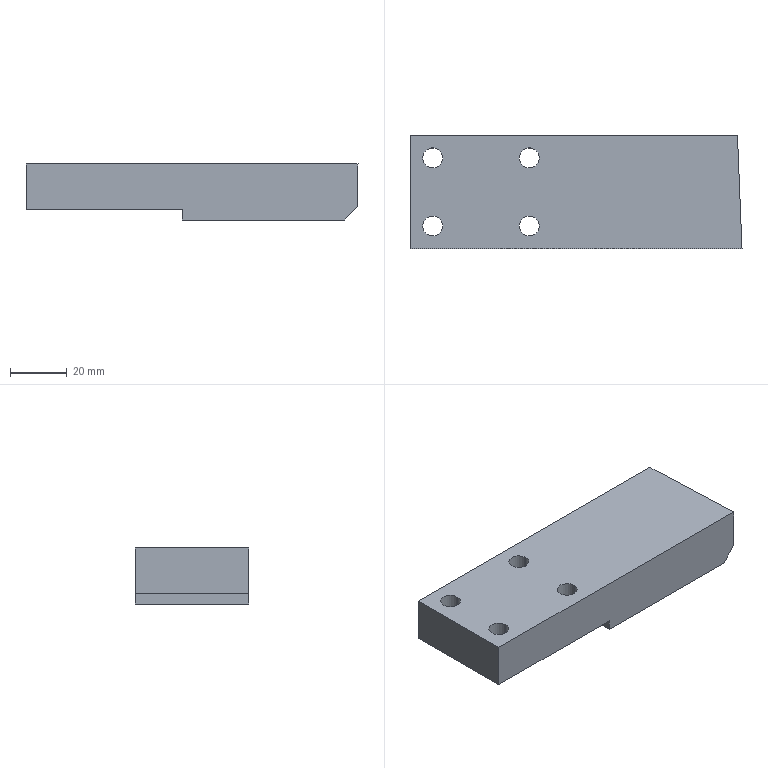Part | STEP file | Positioning_id1530_x_t | 1 solid | 18 faces | box 116.841 x 40 x 19.713 mm | volume 80314 mm3 | cylinder 8 | plane 7 | spline 3 | commonest cylinder face diameters 7 x8